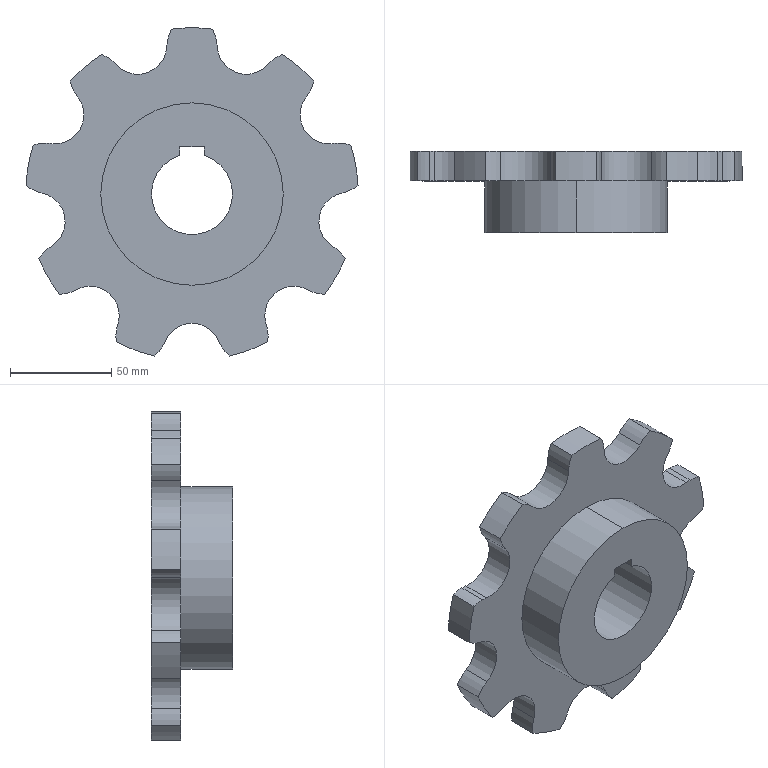Part | STEP file | Produce dryer 9-tooth 40 bore with keyway total width 40 C216AL sprocket | 1 solid | 50 faces | box 163.79 x 40 x 161.93 mm | volume 358621 mm3 | cylinder 44 | plane 6 | commonest cylinder face diameters 38.1 x20 28.58 x12 164 x9 90 x2 40 x1